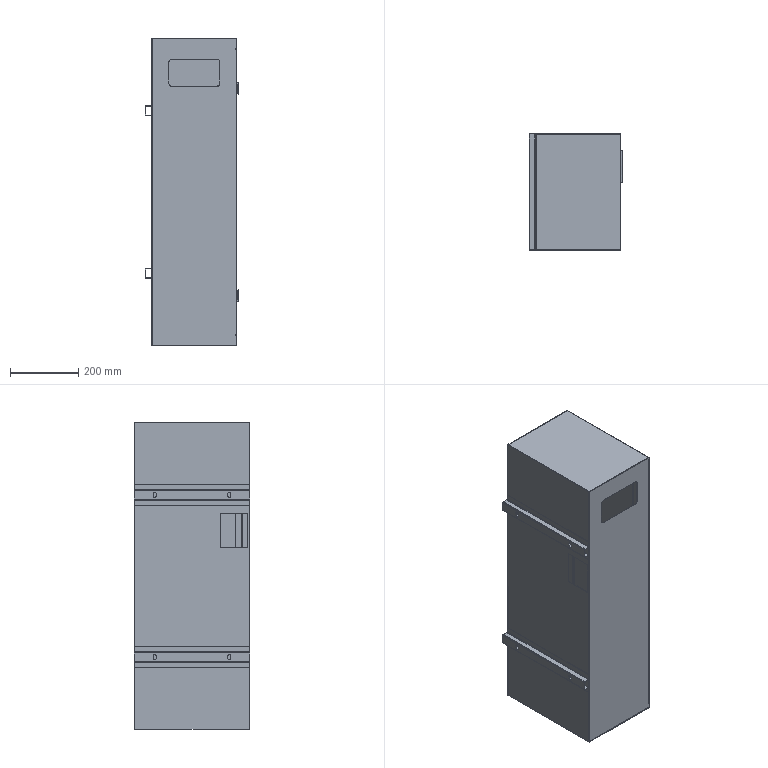Part | SolidWorks | 14 solids | 1407 faces | box 275.9 x 340 x 900 mm | volume 2191586 mm3 | cylinder 589 | plane 558 | spline 186 | torus 62 | sphere 8 | cone 4 | commonest cylinder face diameters 4.8 x240 0.4 x60 2 x38 5 x30 3.2 x28 0.692 x24